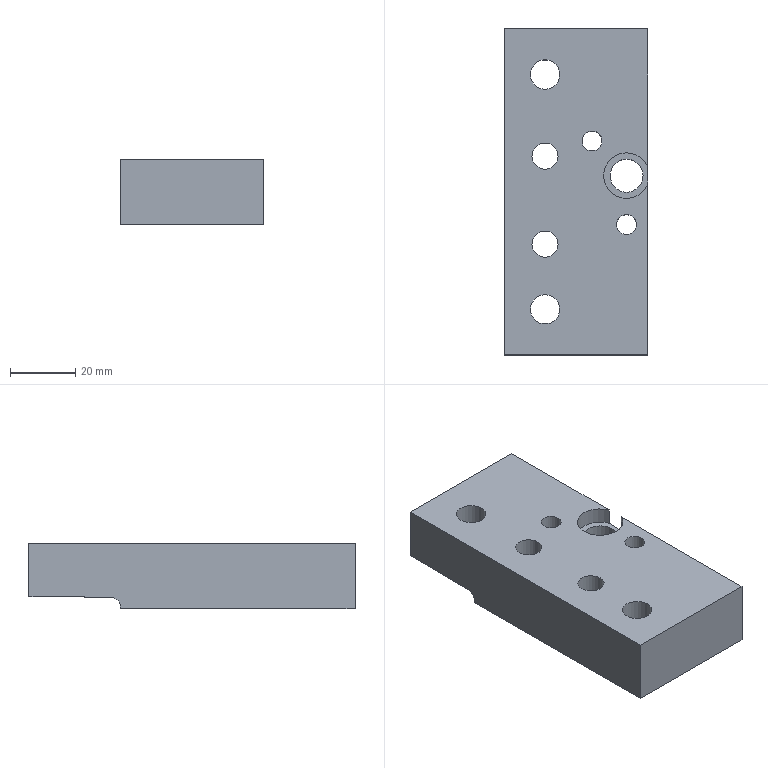Part | STEP file | 410_id618_x_t | 1 solid | 26 faces | box 44 x 100 x 20 mm | volume 73910 mm3 | plane 13 | cylinder 13 | commonest cylinder face diameters 14 x3 6.1 x2 8 x2 9 x2 10 x2 6 x1